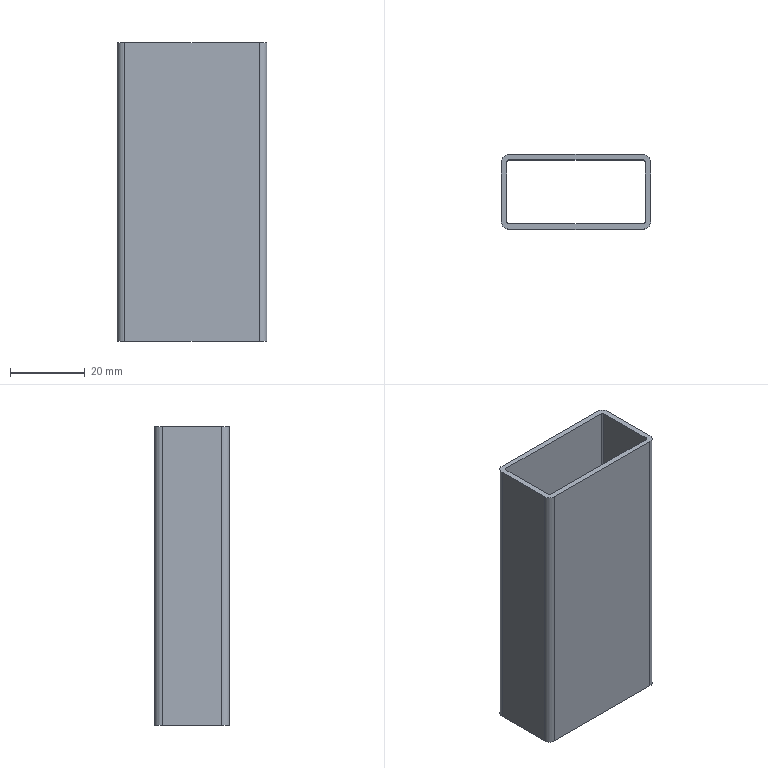Part | STEP file | Q7C0519 | 1 solid | 18 faces | box 40 x 20 x 80 mm | volume 13422 mm3 | plane 10 | cylinder 8 | commonest cylinder face diameters 1 x4 4 x4
STEP:
#1=CARTESIAN_POINT('',(0.,0.,0.));
#2=DIRECTION('',(0.,0.,1.));
#3=DIRECTION('',(1.,0.,0.));
#4=AXIS2_PLACEMENT_3D('',#1,#2,#3);
#5=CARTESIAN_POINT('',(18.,-10.,80.));
#6=VERTEX_POINT('',#5);
#7=CARTESIAN_POINT('',(20.,-8.,80.));
#8=VERTEX_POINT('',#7);
#9=CARTESIAN_POINT('',(18.,-8.,80.));
#10=DIRECTION('',(0.,0.,1.));
#11=DIRECTION('',(1.,0.,0.));
#12=AXIS2_PLACEMENT_3D('',#9,#10,#11);
#13=CIRCLE('',#12,2.);
#14=CARTESIAN_POINT('',(18.,-8.,80.));
#15=DIRECTION('',(0.,0.,1.));
#16=DIRECTION('',(1.,0.,0.));
#17=AXIS2_PLACEMENT_3D('',#14,#15,#16);
#18=PLANE('',#17);
#19=CARTESIAN_POINT('',(0.,0.));
#20=DIRECTION('',(1.,0.));
#21=AXIS2_PLACEMENT_2D('',#19,#20);
#22=CIRCLE('',#21,2.);
#23=(GEOMETRIC_REPRESENTATION_CONTEXT(2)PARAMETRIC_REPRESENTATION_CONTEXT()REPRESENTATION_CONTEXT('',''));
#24=DEFINITIONAL_REPRESENTATION('',(#22),#23);
#25=PCURVE('',#18,#24);
#26=CARTESIAN_POINT('',(18.,-8.,80.));
#27=DIRECTION('',(0.,0.,-1.));
#28=DIRECTION('',(-1.,0.,0.));
#29=AXIS2_PLACEMENT_3D('',#26,#27,#28);
#30=CYLINDRICAL_SURFACE('',#29,2.);
#31=CARTESIAN_POINT('',(9.425,0.));
#32=DIRECTION('',(-1.,0.));
#33=VECTOR('',#32,1.);
#34=LINE('',#31,#33);
#35=(GEOMETRIC_REPRESENTATION_CONTEXT(2)PARAMETRIC_REPRESENTATION_CONTEXT()REPRESENTATION_CONTEXT('',''));
#36=DEFINITIONAL_REPRESENTATION('',(#34),#35);
#37=PCURVE('',#30,#36);
#38=SURFACE_CURVE('',#13,(#25,#37),.PCURVE_S1.);
#39=EDGE_CURVE('',#6,#8,#38,.T.);
#40=ORIENTED_EDGE('',*,*,#39,.T.);
#41=CARTESIAN_POINT('',(20.,8.,80.));
#42=VERTEX_POINT('',#41);
#43=CARTESIAN_POINT('',(20.,8.,80.));
#44=DIRECTION('',(0.,1.,0.));
#45=VECTOR('',#44,1.);
#46=LINE('',#43,#45);
#47=CARTESIAN_POINT('',(2.,16.));
#48=DIRECTION('',(0.,1.));
#49=VECTOR('',#48,1.);
#50=LINE('',#47,#49);
#51=(GEOMETRIC_REPRESENTATION_CONTEXT(2)PARAMETRIC_REPRESENTATION_CONTEXT()REPRESENTATION_CONTEXT('',''));
#52=DEFINITIONAL_REPRESENTATION('',(#50),#51);
#53=PCURVE('',#18,#52);
#54=CARTESIAN_POINT('',(20.,8.,80.));
#55=DIRECTION('',(-1.,0.,0.));
#56=DIRECTION('',(0.,-1.,0.));
#57=AXIS2_PLACEMENT_3D('',#54,#55,#56);
#58=PLANE('',#57);
#59=CARTESIAN_POINT('',(0.,0.));
#60=DIRECTION('',(-1.,0.));
#61=VECTOR('',#60,1.);
#62=LINE('',#59,#61);
#63=(GEOMETRIC_REPRESENTATION_CONTEXT(2)PARAMETRIC_REPRESENTATION_CONTEXT()REPRESENTATION_CONTEXT('',''));
#64=DEFINITIONAL_REPRESENTATION('',(#62),#63);
#65=PCURVE('',#58,#64);
#66=SURFACE_CURVE('',#46,(#53,#65),.PCURVE_S1.);
#67=EDGE_CURVE('',#8,#42,#66,.T.);
#68=ORIENTED_EDGE('',*,*,#67,.T.);
#69=CARTESIAN_POINT('',(18.,10.,80.));
#70=VERTEX_POINT('',#69);
#71=CARTESIAN_POINT('',(18.,8.,80.));
#72=DIRECTION('',(0.,0.,1.));
#73=DIRECTION('',(-1.,0.,0.));
#74=AXIS2_PLACEMENT_3D('',#71,#72,#73);
#75=CIRCLE('',#74,2.);
#76=CARTESIAN_POINT('',(0.,16.));
#77=DIRECTION('',(-1.,0.));
#78=AXIS2_PLACEMENT_2D('',#76,#77);
#79=CIRCLE('',#78,2.);
#80=(GEOMETRIC_REPRESENTATION_CONTEXT(2)PARAMETRIC_REPRESENTATION_CONTEXT()REPRESENTATION_CONTEXT('',''));
#81=DEFINITIONAL_REPRESENTATION('',(#79),#80);
#82=PCURVE('',#18,#81);
#83=CARTESIAN_POINT('',(18.,8.,80.));
#84=DIRECTION('',(0.,0.,-1.));
#85=DIRECTION('',(-1.,0.,0.));
#86=AXIS2_PLACEMENT_3D('',#83,#84,#85);
#87=CYLINDRICAL_SURFACE('',#86,2.);
#88=CARTESIAN_POINT('',(6.283,0.));
#89=DIRECTION('',(-1.,0.));
#90=VECTOR('',#89,1.);
#91=LINE('',#88,#90);
#92=(GEOMETRIC_REPRESENTATION_CONTEXT(2)PARAMETRIC_REPRESENTATION_CONTEXT()REPRESENTATION_CONTEXT('',''));
#93=DEFINITIONAL_REPRESENTATION('',(#91),#92);
#94=PCURVE('',#87,#93);
#95=SURFACE_CURVE('',#75,(#82,#94),.PCURVE_S1.);
#96=EDGE_CURVE('',#42,#70,#95,.T.);
#97=ORIENTED_EDGE('',*,*,#96,.T.);
#98=CARTESIAN_POINT('',(-18.,10.,80.));
#99=VERTEX_POINT('',#98);
#100=CARTESIAN_POINT('',(-18.,10.,80.));
#101=DIRECTION('',(-1.,0.,0.));
#102=VECTOR('',#101,1.);
#103=LINE('',#100,#102);
#104=CARTESIAN_POINT('',(-36.,18.));
#105=DIRECTION('',(-1.,0.));
#106=VECTOR('',#105,1.);
#107=LINE('',#104,#106);
#108=(GEOMETRIC_REPRESENTATION_CONTEXT(2)PARAMETRIC_REPRESENTATION_CONTEXT()REPRESENTATION_CONTEXT('',''));
#109=DEFINITIONAL_REPRESENTATION('',(#107),#108);
#110=PCURVE('',#18,#109);
#111=CARTESIAN_POINT('',(-18.,10.,80.));
#112=DIRECTION('',(0.,-1.,0.));
#113=DIRECTION('',(1.,0.,0.));
#114=AXIS2_PLACEMENT_3D('',#111,#112,#113);
#115=PLANE('',#114);
#116=CARTESIAN_POINT('',(0.,0.));
#117=DIRECTION('',(-1.,0.));
#118=VECTOR('',#117,1.);
#119=LINE('',#116,#118);
#120=(GEOMETRIC_REPRESENTATION_CONTEXT(2)PARAMETRIC_REPRESENTATION_CONTEXT()REPRESENTATION_CONTEXT('',''));
#121=DEFINITIONAL_REPRESENTATION('',(#119),#120);
#122=PCURVE('',#115,#121);
#123=SURFACE_CURVE('',#103,(#110,#122),.PCURVE_S1.);
#124=EDGE_CURVE('',#70,#99,#123,.T.);
#125=ORIENTED_EDGE('',*,*,#124,.T.);
#126=CARTESIAN_POINT('',(-20.,8.,80.));
#127=VERTEX_POINT('',#126);
#128=CARTESIAN_POINT('',(-18.,8.,80.));
#129=DIRECTION('',(0.,0.,1.));
#130=DIRECTION('',(1.,0.,0.));
#131=AXIS2_PLACEMENT_3D('',#128,#129,#130);
#132=CIRCLE('',#131,2.);
#133=CARTESIAN_POINT('',(-36.,16.));
#134=DIRECTION('',(1.,0.));
#135=AXIS2_PLACEMENT_2D('',#133,#134);
#136=CIRCLE('',#135,2.);
#137=(GEOMETRIC_REPRESENTATION_CONTEXT(2)PARAMETRIC_REPRESENTATION_CONTEXT()REPRESENTATION_CONTEXT('',''));
#138=DEFINITIONAL_REPRESENTATION('',(#136),#137);
#139=PCURVE('',#18,#138);
#140=CARTESIAN_POINT('',(-18.,8.,80.));
#141=DIRECTION('',(0.,0.,-1.));
#142=DIRECTION('',(-1.,0.,0.));
#143=AXIS2_PLACEMENT_3D('',#140,#141,#142);
#144=CYLINDRICAL_SURFACE('',#143,2.);
#145=CARTESIAN_POINT('',(3.142,0.));
#146=DIRECTION('',(-1.,0.));
#147=VECTOR('',#146,1.);
#148=LINE('',#145,#147);
#149=(GEOMETRIC_REPRESENTATION_CONTEXT(2)PARAMETRIC_REPRESENTATION_CONTEXT()REPRESENTATION_CONTEXT('',''));
#150=DEFINITIONAL_REPRESENTATION('',(#148),#149);
#151=PCURVE('',#144,#150);
#152=SURFACE_CURVE('',#132,(#139,#151),.PCURVE_S1.);
#153=EDGE_CURVE('',#99,#127,#152,.T.);
#154=ORIENTED_EDGE('',*,*,#153,.T.);
#155=CARTESIAN_POINT('',(-20.,-8.,80.));
#156=VERTEX_POINT('',#155);
#157=CARTESIAN_POINT('',(-20.,8.,80.));
#158=DIRECTION('',(0.,-1.,0.));
#159=VECTOR('',#158,1.);
#160=LINE('',#157,#159);
#161=CARTESIAN_POINT('',(-38.,16.));
#162=DIRECTION('',(0.,-1.));
#163=VECTOR('',#162,1.);
#164=LINE('',#161,#163);
#165=(GEOMETRIC_REPRESENTATION_CONTEXT(2)PARAMETRIC_REPRESENTATION_CONTEXT()REPRESENTATION_CONTEXT('',''));
#166=DEFINITIONAL_REPRESENTATION('',(#164),#165);
#167=PCURVE('',#18,#166);
#168=CARTESIAN_POINT('',(-20.,8.,80.));
#169=DIRECTION('',(1.,0.,0.));
#170=DIRECTION('',(0.,1.,0.));
#171=AXIS2_PLACEMENT_3D('',#168,#169,#170);
#172=PLANE('',#171);
#173=CARTESIAN_POINT('',(0.,0.));
#174=DIRECTION('',(-1.,0.));
#175=VECTOR('',#174,1.);
#176=LINE('',#173,#175);
#177=(GEOMETRIC_REPRESENTATION_CONTEXT(2)PARAMETRIC_REPRESENTATION_CONTEXT()REPRESENTATION_CONTEXT('',''));
#178=DEFINITIONAL_REPRESENTATION('',(#176),#177);
#179=PCURVE('',#172,#178);
#180=SURFACE_CURVE('',#160,(#167,#179),.PCURVE_S1.);
#181=EDGE_CURVE('',#127,#156,#180,.T.);
#182=ORIENTED_EDGE('',*,*,#181,.T.);
#183=CARTESIAN_POINT('',(-18.,-10.,80.));
#184=VERTEX_POINT('',#183);
#185=CARTESIAN_POINT('',(-18.,-8.,80.));
#186=DIRECTION('',(0.,0.,1.));
#187=DIRECTION('',(1.,0.,0.));
#188=AXIS2_PLACEMENT_3D('',#185,#186,#187);
#189=CIRCLE('',#188,2.);
#190=CARTESIAN_POINT('',(-36.,0.));
#191=DIRECTION('',(1.,0.));
#192=AXIS2_PLACEMENT_2D('',#190,#191);
#193=CIRCLE('',#192,2.);
#194=(GEOMETRIC_REPRESENTATION_CONTEXT(2)PARAMETRIC_REPRESENTATION_CONTEXT()REPRESENTATION_CONTEXT('',''));
#195=DEFINITIONAL_REPRESENTATION('',(#193),#194);
#196=PCURVE('',#18,#195);
#197=CARTESIAN_POINT('',(-18.,-8.,80.));
#198=DIRECTION('',(0.,0.,-1.));
#199=DIRECTION('',(-1.,0.,0.));
#200=AXIS2_PLACEMENT_3D('',#197,#198,#199);
#201=CYLINDRICAL_SURFACE('',#200,2.);
#202=CARTESIAN_POINT('',(9.425,0.));
#203=DIRECTION('',(-1.,0.));
#204=VECTOR('',#203,1.);
#205=LINE('',#202,#204);
#206=(GEOMETRIC_REPRESENTATION_CONTEXT(2)PARAMETRIC_REPRESENTATION_CONTEXT()REPRESENTATION_CONTEXT('',''));
#207=DEFINITIONAL_REPRESENTATION('',(#205),#206);
#208=PCURVE('',#201,#207);
#209=SURFACE_CURVE('',#189,(#196,#208),.PCURVE_S1.);
#210=EDGE_CURVE('',#156,#184,#209,.T.);
#211=ORIENTED_EDGE('',*,*,#210,.T.);
#212=CARTESIAN_POINT('',(-18.,-10.,80.));
#213=DIRECTION('',(1.,0.,0.));
#214=VECTOR('',#213,1.);
#215=LINE('',#212,#214);
#216=CARTESIAN_POINT('',(-36.,-2.));
#217=DIRECTION('',(1.,0.));
#218=VECTOR('',#217,1.);
#219=LINE('',#216,#218);
#220=(GEOMETRIC_REPRESENTATION_CONTEXT(2)PARAMETRIC_REPRESENTATION_CONTEXT()REPRESENTATION_CONTEXT('',''));
#221=DEFINITIONAL_REPRESENTATION('',(#219),#220);
#222=PCURVE('',#18,#221);
#223=CARTESIAN_POINT('',(-18.,-10.,80.));
#224=DIRECTION('',(0.,1.,0.));
#225=DIRECTION('',(0.,0.,1.));
#226=AXIS2_PLACEMENT_3D('',#223,#224,#225);
#227=PLANE('',#226);
#228=CARTESIAN_POINT('',(0.,0.));
#229=DIRECTION('',(0.,1.));
#230=VECTOR('',#229,1.);
#231=LINE('',#228,#230);
#232=(GEOMETRIC_REPRESENTATION_CONTEXT(2)PARAMETRIC_REPRESENTATION_CONTEXT()REPRESENTATION_CONTEXT('',''));
#233=DEFINITIONAL_REPRESENTATION('',(#231),#232);
#234=PCURVE('',#227,#233);
#235=SURFACE_CURVE('',#215,(#222,#234),.PCURVE_S1.);
#236=EDGE_CURVE('',#184,#6,#235,.T.);
#237=ORIENTED_EDGE('',*,*,#236,.T.);
#238=EDGE_LOOP('',(#40,#68,#97,#125,#154,#182,#211,#237));
#239=FACE_BOUND('',#238,.T.);
#240=CARTESIAN_POINT('',(18.,8.5,80.));
#241=VERTEX_POINT('',#240);
#242=CARTESIAN_POINT('',(-18.,8.5,80.));
#243=VERTEX_POINT('',#242);
#244=CARTESIAN_POINT('',(-18.,8.5,80.));
#245=DIRECTION('',(-1.,0.,0.));
#246=VECTOR('',#245,1.);
#247=LINE('',#244,#246);
#248=CARTESIAN_POINT('',(-36.,16.5));
#249=DIRECTION('',(-1.,0.));
#250=VECTOR('',#249,1.);
#251=LINE('',#248,#250);
#252=(GEOMETRIC_REPRESENTATION_CONTEXT(2)PARAMETRIC_REPRESENTATION_CONTEXT()REPRESENTATION_CONTEXT('',''));
#253=DEFINITIONAL_REPRESENTATION('',(#251),#252);
#254=PCURVE('',#18,#253);
#255=CARTESIAN_POINT('',(-18.,8.5,80.));
#256=DIRECTION('',(0.,-1.,0.));
#257=DIRECTION('',(1.,0.,0.));
#258=AXIS2_PLACEMENT_3D('',#255,#256,#257);
#259=PLANE('',#258);
#260=CARTESIAN_POINT('',(0.,0.));
#261=DIRECTION('',(-1.,0.));
#262=VECTOR('',#261,1.);
#263=LINE('',#260,#262);
#264=(GEOMETRIC_REPRESENTATION_CONTEXT(2)PARAMETRIC_REPRESENTATION_CONTEXT()REPRESENTATION_CONTEXT('',''));
#265=DEFINITIONAL_REPRESENTATION('',(#263),#264);
#266=PCURVE('',#259,#265);
#267=SURFACE_CURVE('',#247,(#254,#266),.PCURVE_S1.);
#268=EDGE_CURVE('',#241,#243,#267,.T.);
#269=ORIENTED_EDGE('',*,*,#268,.F.);
#270=CARTESIAN_POINT('',(18.5,8.,80.));
#271=VERTEX_POINT('',#270);
#272=CARTESIAN_POINT('',(18.,8.,80.));
#273=DIRECTION('',(0.,0.,1.));
#274=DIRECTION('',(-1.,0.,0.));
#275=AXIS2_PLACEMENT_3D('',#272,#273,#274);
#276=CIRCLE('',#275,0.5);
#277=CARTESIAN_POINT('',(0.,16.));
#278=DIRECTION('',(-1.,0.));
#279=AXIS2_PLACEMENT_2D('',#277,#278);
#280=CIRCLE('',#279,0.5);
#281=(GEOMETRIC_REPRESENTATION_CONTEXT(2)PARAMETRIC_REPRESENTATION_CONTEXT()REPRESENTATION_CONTEXT('',''));
#282=DEFINITIONAL_REPRESENTATION('',(#280),#281);
#283=PCURVE('',#18,#282);
#284=CARTESIAN_POINT('',(18.,8.,80.));
#285=DIRECTION('',(0.,0.,-1.));
#286=DIRECTION('',(-1.,0.,0.));
#287=AXIS2_PLACEMENT_3D('',#284,#285,#286);
#288=CYLINDRICAL_SURFACE('',#287,0.5);
#289=CARTESIAN_POINT('',(6.283,0.));
#290=DIRECTION('',(-1.,0.));
#291=VECTOR('',#290,1.);
#292=LINE('',#289,#291);
#293=(GEOMETRIC_REPRESENTATION_CONTEXT(2)PARAMETRIC_REPRESENTATION_CONTEXT()REPRESENTATION_CONTEXT('',''));
#294=DEFINITIONAL_REPRESENTATION('',(#292),#293);
#295=PCURVE('',#288,#294);
#296=SURFACE_CURVE('',#276,(#283,#295),.PCURVE_S1.);
#297=EDGE_CURVE('',#271,#241,#296,.T.);
#298=ORIENTED_EDGE('',*,*,#297,.F.);
#299=CARTESIAN_POINT('',(18.5,-8.,80.));
#300=VERTEX_POINT('',#299);
#301=CARTESIAN_POINT('',(18.5,8.,80.));
#302=DIRECTION('',(0.,1.,0.));
#303=VECTOR('',#302,1.);
#304=LINE('',#301,#303);
#305=CARTESIAN_POINT('',(0.5,16.));
#306=DIRECTION('',(0.,1.));
#307=VECTOR('',#306,1.);
#308=LINE('',#305,#307);
#309=(GEOMETRIC_REPRESENTATION_CONTEXT(2)PARAMETRIC_REPRESENTATION_CONTEXT()REPRESENTATION_CONTEXT('',''));
#310=DEFINITIONAL_REPRESENTATION('',(#308),#309);
#311=PCURVE('',#18,#310);
#312=CARTESIAN_POINT('',(18.5,8.,80.));
#313=DIRECTION('',(-1.,0.,0.));
#314=DIRECTION('',(0.,0.,1.));
#315=AXIS2_PLACEMENT_3D('',#312,#313,#314);
#316=PLANE('',#315);
#317=CARTESIAN_POINT('',(0.,0.));
#318=DIRECTION('',(0.,1.));
#319=VECTOR('',#318,1.);
#320=LINE('',#317,#319);
#321=(GEOMETRIC_REPRESENTATION_CONTEXT(2)PARAMETRIC_REPRESENTATION_CONTEXT()REPRESENTATION_CONTEXT('',''));
#322=DEFINITIONAL_REPRESENTATION('',(#320),#321);
#323=PCURVE('',#316,#322);
#324=SURFACE_CURVE('',#304,(#311,#323),.PCURVE_S1.);
#325=EDGE_CURVE('',#300,#271,#324,.T.);
#326=ORIENTED_EDGE('',*,*,#325,.F.);
#327=CARTESIAN_POINT('',(18.,-8.5,80.));
#328=VERTEX_POINT('',#327);
#329=CARTESIAN_POINT('',(18.,-8.,80.));
#330=DIRECTION('',(0.,0.,1.));
#331=DIRECTION('',(1.,0.,0.));
#332=AXIS2_PLACEMENT_3D('',#329,#330,#331);
#333=CIRCLE('',#332,0.5);
#334=CARTESIAN_POINT('',(0.,0.));
#335=DIRECTION('',(1.,0.));
#336=AXIS2_PLACEMENT_2D('',#334,#335);
#337=CIRCLE('',#336,0.5);
#338=(GEOMETRIC_REPRESENTATION_CONTEXT(2)PARAMETRIC_REPRESENTATION_CONTEXT()REPRESENTATION_CONTEXT('',''));
#339=DEFINITIONAL_REPRESENTATION('',(#337),#338);
#340=PCURVE('',#18,#339);
#341=CARTESIAN_POINT('',(18.,-8.,80.));
#342=DIRECTION('',(0.,0.,-1.));
#343=DIRECTION('',(-1.,0.,0.));
#344=AXIS2_PLACEMENT_3D('',#341,#342,#343);
#345=CYLINDRICAL_SURFACE('',#344,0.5);
#346=CARTESIAN_POINT('',(9.425,0.));
#347=DIRECTION('',(-1.,0.));
#348=VECTOR('',#347,1.);
#349=LINE('',#346,#348);
#350=(GEOMETRIC_REPRESENTATION_CONTEXT(2)PARAMETRIC_REPRESENTATION_CONTEXT()REPRESENTATION_CONTEXT('',''));
#351=DEFINITIONAL_REPRESENTATION('',(#349),#350);
#352=PCURVE('',#345,#351);
#353=SURFACE_CURVE('',#333,(#340,#352),.PCURVE_S1.);
#354=EDGE_CURVE('',#328,#300,#353,.T.);
#355=ORIENTED_EDGE('',*,*,#354,.F.);
#356=CARTESIAN_POINT('',(-18.,-8.5,80.));
#357=VERTEX_POINT('',#356);
#358=CARTESIAN_POINT('',(-18.,-8.5,80.));
#359=DIRECTION('',(1.,0.,0.));
#360=VECTOR('',#359,1.);
#361=LINE('',#358,#360);
#362=CARTESIAN_POINT('',(-36.,-0.5));
#363=DIRECTION('',(1.,0.));
#364=VECTOR('',#363,1.);
#365=LINE('',#362,#364);
#366=(GEOMETRIC_REPRESENTATION_CONTEXT(2)PARAMETRIC_REPRESENTATION_CONTEXT()REPRESENTATION_CONTEXT('',''));
#367=DEFINITIONAL_REPRESENTATION('',(#365),#366);
#368=PCURVE('',#18,#367);
#369=CARTESIAN_POINT('',(-18.,-8.5,80.));
#370=DIRECTION('',(0.,1.,0.));
#371=DIRECTION('',(-1.,0.,0.));
#372=AXIS2_PLACEMENT_3D('',#369,#370,#371);
#373=PLANE('',#372);
#374=CARTESIAN_POINT('',(0.,0.));
#375=DIRECTION('',(-1.,0.));
#376=VECTOR('',#375,1.);
#377=LINE('',#374,#376);
#378=(GEOMETRIC_REPRESENTATION_CONTEXT(2)PARAMETRIC_REPRESENTATION_CONTEXT()REPRESENTATION_CONTEXT('',''));
#379=DEFINITIONAL_REPRESENTATION('',(#377),#378);
#380=PCURVE('',#373,#379);
#381=SURFACE_CURVE('',#361,(#368,#380),.PCURVE_S1.);
#382=EDGE_CURVE('',#357,#328,#381,.T.);
#383=ORIENTED_EDGE('',*,*,#382,.F.);
#384=CARTESIAN_POINT('',(-18.5,-8.,80.));
#385=VERTEX_POINT('',#384);
#386=CARTESIAN_POINT('',(-18.,-8.,80.));
#387=DIRECTION('',(0.,0.,1.));
#388=DIRECTION('',(1.,0.,0.));
#389=AXIS2_PLACEMENT_3D('',#386,#387,#388);
#390=CIRCLE('',#389,0.5);
#391=CARTESIAN_POINT('',(-36.,0.));
#392=DIRECTION('',(1.,0.));
#393=AXIS2_PLACEMENT_2D('',#391,#392);
#394=CIRCLE('',#393,0.5);
#395=(GEOMETRIC_REPRESENTATION_CONTEXT(2)PARAMETRIC_REPRESENTATION_CONTEXT()REPRESENTATION_CONTEXT('',''));
#396=DEFINITIONAL_REPRESENTATION('',(#394),#395);
#397=PCURVE('',#18,#396);
#398=CARTESIAN_POINT('',(-18.,-8.,80.));
#399=DIRECTION('',(0.,0.,-1.));
#400=DIRECTION('',(-1.,0.,0.));
#401=AXIS2_PLACEMENT_3D('',#398,#399,#400);
#402=CYLINDRICAL_SURFACE('',#401,0.5);
#403=CARTESIAN_POINT('',(9.425,0.));
#404=DIRECTION('',(-1.,0.));
#405=VECTOR('',#404,1.);
#406=LINE('',#403,#405);
#407=(GEOMETRIC_REPRESENTATION_CONTEXT(2)PARAMETRIC_REPRESENTATION_CONTEXT()REPRESENTATION_CONTEXT('',''));
#408=DEFINITIONAL_REPRESENTATION('',(#406),#407);
#409=PCURVE('',#402,#408);
#410=SURFACE_CURVE('',#390,(#397,#409),.PCURVE_S1.);
#411=EDGE_CURVE('',#385,#357,#410,.T.);
#412=ORIENTED_EDGE('',*,*,#411,.F.);
#413=CARTESIAN_POINT('',(-18.5,8.,80.));
#414=VERTEX_POINT('',#413);
#415=CARTESIAN_POINT('',(-18.5,8.,80.));
#416=DIRECTION('',(0.,-1.,0.));
#417=VECTOR('',#416,1.);
#418=LINE('',#415,#417);
#419=CARTESIAN_POINT('',(-36.5,16.));
#420=DIRECTION('',(0.,-1.));
#421=VECTOR('',#420,1.);
#422=LINE('',#419,#421);
#423=(GEOMETRIC_REPRESENTATION_CONTEXT(2)PARAMETRIC_REPRESENTATION_CONTEXT()REPRESENTATION_CONTEXT('',''));
#424=DEFINITIONAL_REPRESENTATION('',(#422),#423);
#425=PCURVE('',#18,#424);
#426=CARTESIAN_POINT('',(-18.5,8.,80.));
#427=DIRECTION('',(1.,0.,0.));
#428=DIRECTION('',(0.,0.,-1.));
#429=AXIS2_PLACEMENT_3D('',#426,#427,#428);
#430=PLANE('',#429);
#431=CARTESIAN_POINT('',(0.,0.));
#432=DIRECTION('',(0.,-1.));
#433=VECTOR('',#432,1.);
#434=LINE('',#431,#433);
#435=(GEOMETRIC_REPRESENTATION_CONTEXT(2)PARAMETRIC_REPRESENTATION_CONTEXT()REPRESENTATION_CONTEXT('',''));
#436=DEFINITIONAL_REPRESENTATION('',(#434),#435);
#437=PCURVE('',#430,#436);
#438=SURFACE_CURVE('',#418,(#425,#437),.PCURVE_S1.);
#439=EDGE_CURVE('',#414,#385,#438,.T.);
#440=ORIENTED_EDGE('',*,*,#439,.F.);
#441=CARTESIAN_POINT('',(-18.,8.,80.));
#442=DIRECTION('',(0.,0.,1.));
#443=DIRECTION('',(1.,0.,0.));
#444=AXIS2_PLACEMENT_3D('',#441,#442,#443);
#445=CIRCLE('',#444,0.5);
#446=CARTESIAN_POINT('',(-36.,16.));
#447=DIRECTION('',(1.,0.));
#448=AXIS2_PLACEMENT_2D('',#446,#447);
#449=CIRCLE('',#448,0.5);
#450=(GEOMETRIC_REPRESENTATION_CONTEXT(2)PARAMETRIC_REPRESENTATION_CONTEXT()REPRESENTATION_CONTEXT('',''));
#451=DEFINITIONAL_REPRESENTATION('',(#449),#450);
#452=PCURVE('',#18,#451);
#453=CARTESIAN_POINT('',(-18.,8.,80.));
#454=DIRECTION('',(0.,0.,-1.));
#455=DIRECTION('',(-1.,0.,0.));
#456=AXIS2_PLACEMENT_3D('',#453,#454,#455);
#457=CYLINDRICAL_SURFACE('',#456,0.5);
#458=CARTESIAN_POINT('',(3.142,0.));
#459=DIRECTION('',(-1.,0.));
#460=VECTOR('',#459,1.);
#461=LINE('',#458,#460);
#462=(GEOMETRIC_REPRESENTATION_CONTEXT(2)PARAMETRIC_REPRESENTATION_CONTEXT()REPRESENTATION_CONTEXT('',''));
#463=DEFINITIONAL_REPRESENTATION('',(#461),#462);
#464=PCURVE('',#457,#463);
#465=SURFACE_CURVE('',#445,(#452,#464),.PCURVE_S1.);
#466=EDGE_CURVE('',#243,#414,#465,.T.);
#467=ORIENTED_EDGE('',*,*,#466,.F.);
#468=EDGE_LOOP('',(#269,#298,#326,#355,#383,#412,#440,#467));
#469=FACE_BOUND('',#468,.T.);
#470=ADVANCED_FACE('',(#239,#469),#18,.T.);
#471=CARTESIAN_POINT('',(18.,-10.,0.));
#472=VERTEX_POINT('',#471);
#473=CARTESIAN_POINT('',(20.,-8.,0.));
#474=VERTEX_POINT('',#473);
#475=CARTESIAN_POINT('',(18.,-8.,0.));
#476=DIRECTION('',(0.,0.,1.));
#477=DIRECTION('',(1.,0.,0.));
#478=AXIS2_PLACEMENT_3D('',#475,#476,#477);
#479=CIRCLE('',#478,2.);
#480=CARTESIAN_POINT('',(18.,-8.,0.));
#481=DIRECTION('',(0.,0.,1.));
#482=DIRECTION('',(1.,0.,0.));
#483=AXIS2_PLACEMENT_3D('',#480,#481,#482);
#484=PLANE('',#483);
#485=CARTESIAN_POINT('',(0.,0.));
#486=DIRECTION('',(1.,0.));
#487=AXIS2_PLACEMENT_2D('',#485,#486);
#488=CIRCLE('',#487,2.);
#489=(GEOMETRIC_REPRESENTATION_CONTEXT(2)PARAMETRIC_REPRESENTATION_CONTEXT()REPRESENTATION_CONTEXT('',''));
#490=DEFINITIONAL_REPRESENTATION('',(#488),#489);
#491=PCURVE('',#484,#490);
#492=CARTESIAN_POINT('',(9.425,80.));
#493=DIRECTION('',(-1.,0.));
#494=VECTOR('',#493,1.);
#495=LINE('',#492,#494);
#496=(GEOMETRIC_REPRESENTATION_CONTEXT(2)PARAMETRIC_REPRESENTATION_CONTEXT()REPRESENTATION_CONTEXT('',''));
#497=DEFINITIONAL_REPRESENTATION('',(#495),#496);
#498=PCURVE('',#30,#497);
#499=SURFACE_CURVE('',#479,(#491,#498),.PCURVE_S1.);
#500=EDGE_CURVE('',#472,#474,#499,.T.);
#501=ORIENTED_EDGE('',*,*,#500,.F.);
#502=CARTESIAN_POINT('',(-18.,-10.,0.));
#503=VERTEX_POINT('',#502);
#504=CARTESIAN_POINT('',(-18.,-10.,0.));
#505=DIRECTION('',(1.,0.,0.));
#506=VECTOR('',#505,1.);
#507=LINE('',#504,#506);
#508=CARTESIAN_POINT('',(-36.,-2.));
#509=DIRECTION('',(1.,0.));
#510=VECTOR('',#509,1.);
#511=LINE('',#508,#510);
#512=(GEOMETRIC_REPRESENTATION_CONTEXT(2)PARAMETRIC_REPRESENTATION_CONTEXT()REPRESENTATION_CONTEXT('',''));
#513=DEFINITIONAL_REPRESENTATION('',(#511),#512);
#514=PCURVE('',#484,#513);
#515=CARTESIAN_POINT('',(-80.,0.));
#516=DIRECTION('',(0.,1.));
#517=VECTOR('',#516,1.);
#518=LINE('',#515,#517);
#519=(GEOMETRIC_REPRESENTATION_CONTEXT(2)PARAMETRIC_REPRESENTATION_CONTEXT()REPRESENTATION_CONTEXT('',''));
#520=DEFINITIONAL_REPRESENTATION('',(#518),#519);
#521=PCURVE('',#227,#520);
#522=SURFACE_CURVE('',#507,(#514,#521),.PCURVE_S1.);
#523=EDGE_CURVE('',#503,#472,#522,.T.);
#524=ORIENTED_EDGE('',*,*,#523,.F.);
#525=CARTESIAN_POINT('',(-20.,-8.,0.));
#526=VERTEX_POINT('',#525);
#527=CARTESIAN_POINT('',(-18.,-8.,0.));
#528=DIRECTION('',(0.,0.,1.));
#529=DIRECTION('',(1.,0.,0.));
#530=AXIS2_PLACEMENT_3D('',#527,#528,#529);
#531=CIRCLE('',#530,2.);
#532=CARTESIAN_POINT('',(-36.,0.));
#533=DIRECTION('',(1.,0.));
#534=AXIS2_PLACEMENT_2D('',#532,#533);
#535=CIRCLE('',#534,2.);
#536=(GEOMETRIC_REPRESENTATION_CONTEXT(2)PARAMETRIC_REPRESENTATION_CONTEXT()REPRESENTATION_CONTEXT('',''));
#537=DEFINITIONAL_REPRESENTATION('',(#535),#536);
#538=PCURVE('',#484,#537);
#539=CARTESIAN_POINT('',(9.425,80.));
#540=DIRECTION('',(-1.,0.));
#541=VECTOR('',#540,1.);
#542=LINE('',#539,#541);
#543=(GEOMETRIC_REPRESENTATION_CONTEXT(2)PARAMETRIC_REPRESENTATION_CONTEXT()REPRESENTATION_CONTEXT('',''));
#544=DEFINITIONAL_REPRESENTATION('',(#542),#543);
#545=PCURVE('',#201,#544);
#546=SURFACE_CURVE('',#531,(#538,#545),.PCURVE_S1.);
#547=EDGE_CURVE('',#526,#503,#546,.T.);
#548=ORIENTED_EDGE('',*,*,#547,.F.);
#549=CARTESIAN_POINT('',(-20.,8.,0.));
#550=VERTEX_POINT('',#549);
#551=CARTESIAN_POINT('',(-20.,8.,0.));
#552=DIRECTION('',(0.,-1.,0.));
#553=VECTOR('',#552,1.);
#554=LINE('',#551,#553);
#555=CARTESIAN_POINT('',(-38.,16.));
#556=DIRECTION('',(0.,-1.));
#557=VECTOR('',#556,1.);
#558=LINE('',#555,#557);
#559=(GEOMETRIC_REPRESENTATION_CONTEXT(2)PARAMETRIC_REPRESENTATION_CONTEXT()REPRESENTATION_CONTEXT('',''));
#560=DEFINITIONAL_REPRESENTATION('',(#558),#559);
#561=PCURVE('',#484,#560);
#562=CARTESIAN_POINT('',(0.,-80.));
#563=DIRECTION('',(-1.,0.));
#564=VECTOR('',#563,1.);
#565=LINE('',#562,#564);
#566=(GEOMETRIC_REPRESENTATION_CONTEXT(2)PARAMETRIC_REPRESENTATION_CONTEXT()REPRESENTATION_CONTEXT('',''));
#567=DEFINITIONAL_REPRESENTATION('',(#565),#566);
#568=PCURVE('',#172,#567);
#569=SURFACE_CURVE('',#554,(#561,#568),.PCURVE_S1.);
#570=EDGE_CURVE('',#550,#526,#569,.T.);
#571=ORIENTED_EDGE('',*,*,#570,.F.);
#572=CARTESIAN_POINT('',(-18.,10.,0.));
#573=VERTEX_POINT('',#572);
#574=CARTESIAN_POINT('',(-18.,8.,0.));
#575=DIRECTION('',(0.,0.,1.));
#576=DIRECTION('',(1.,0.,0.));
#577=AXIS2_PLACEMENT_3D('',#574,#575,#576);
#578=CIRCLE('',#577,2.);
#579=CARTESIAN_POINT('',(-36.,16.));
#580=DIRECTION('',(1.,0.));
#581=AXIS2_PLACEMENT_2D('',#579,#580);
#582=CIRCLE('',#581,2.);
#583=(GEOMETRIC_REPRESENTATION_CONTEXT(2)PARAMETRIC_REPRESENTATION_CONTEXT()REPRESENTATION_CONTEXT('',''));
#584=DEFINITIONAL_REPRESENTATION('',(#582),#583);
#585=PCURVE('',#484,#584);
#586=CARTESIAN_POINT('',(3.142,80.));
#587=DIRECTION('',(-1.,0.));
#588=VECTOR('',#587,1.);
#589=LINE('',#586,#588);
#590=(GEOMETRIC_REPRESENTATION_CONTEXT(2)PARAMETRIC_REPRESENTATION_CONTEXT()REPRESENTATION_CONTEXT('',''));
#591=DEFINITIONAL_REPRESENTATION('',(#589),#590);
#592=PCURVE('',#144,#591);
#593=SURFACE_CURVE('',#578,(#585,#592),.PCURVE_S1.);
#594=EDGE_CURVE('',#573,#550,#593,.T.);
#595=ORIENTED_EDGE('',*,*,#594,.F.);
#596=CARTESIAN_POINT('',(18.,10.,0.));
#597=VERTEX_POINT('',#596);
#598=CARTESIAN_POINT('',(-18.,10.,0.));
#599=DIRECTION('',(-1.,0.,0.));
#600=VECTOR('',#599,1.);
#601=LINE('',#598,#600);
#602=CARTESIAN_POINT('',(-36.,18.));
#603=DIRECTION('',(-1.,0.));
#604=VECTOR('',#603,1.);
#605=LINE('',#602,#604);
#606=(GEOMETRIC_REPRESENTATION_CONTEXT(2)PARAMETRIC_REPRESENTATION_CONTEXT()REPRESENTATION_CONTEXT('',''));
#607=DEFINITIONAL_REPRESENTATION('',(#605),#606);
#608=PCURVE('',#484,#607);
#609=CARTESIAN_POINT('',(0.,-80.));
#610=DIRECTION('',(-1.,0.));
#611=VECTOR('',#610,1.);
#612=LINE('',#609,#611);
#613=(GEOMETRIC_REPRESENTATION_CONTEXT(2)PARAMETRIC_REPRESENTATION_CONTEXT()REPRESENTATION_CONTEXT('',''));
#614=DEFINITIONAL_REPRESENTATION('',(#612),#613);
#615=PCURVE('',#115,#614);
#616=SURFACE_CURVE('',#601,(#608,#615),.PCURVE_S1.);
#617=EDGE_CURVE('',#597,#573,#616,.T.);
#618=ORIENTED_EDGE('',*,*,#617,.F.);
#619=CARTESIAN_POINT('',(20.,8.,0.));
#620=VERTEX_POINT('',#619);
#621=CARTESIAN_POINT('',(18.,8.,0.));
#622=DIRECTION('',(0.,0.,1.));
#623=DIRECTION('',(-1.,0.,0.));
#624=AXIS2_PLACEMENT_3D('',#621,#622,#623);
#625=CIRCLE('',#624,2.);
#626=CARTESIAN_POINT('',(0.,16.));
#627=DIRECTION('',(-1.,0.));
#628=AXIS2_PLACEMENT_2D('',#626,#627);
#629=CIRCLE('',#628,2.);
#630=(GEOMETRIC_REPRESENTATION_CONTEXT(2)PARAMETRIC_REPRESENTATION_CONTEXT()REPRESENTATION_CONTEXT('',''));
#631=DEFINITIONAL_REPRESENTATION('',(#629),#630);
#632=PCURVE('',#484,#631);
#633=CARTESIAN_POINT('',(6.283,80.));
#634=DIRECTION('',(-1.,0.));
#635=VECTOR('',#634,1.);
#636=LINE('',#633,#635);
#637=(GEOMETRIC_REPRESENTATION_CONTEXT(2)PARAMETRIC_REPRESENTATION_CONTEXT()REPRESENTATION_CONTEXT('',''));
#638=DEFINITIONAL_REPRESENTATION('',(#636),#637);
#639=PCURVE('',#87,#638);
#640=SURFACE_CURVE('',#625,(#632,#639),.PCURVE_S1.);
#641=EDGE_CURVE('',#620,#597,#640,.T.);
#642=ORIENTED_EDGE('',*,*,#641,.F.);
#643=CARTESIAN_POINT('',(20.,8.,0.));
#644=DIRECTION('',(0.,1.,0.));
#645=VECTOR('',#644,1.);
#646=LINE('',#643,#645);
#647=CARTESIAN_POINT('',(2.,16.));
#648=DIRECTION('',(0.,1.));
#649=VECTOR('',#648,1.);
#650=LINE('',#647,#649);
#651=(GEOMETRIC_REPRESENTATION_CONTEXT(2)PARAMETRIC_REPRESENTATION_CONTEXT()REPRESENTATION_CONTEXT('',''));
#652=DEFINITIONAL_REPRESENTATION('',(#650),#651);
#653=PCURVE('',#484,#652);
#654=CARTESIAN_POINT('',(0.,-80.));
#655=DIRECTION('',(-1.,0.));
#656=VECTOR('',#655,1.);
#657=LINE('',#654,#656);
#658=(GEOMETRIC_REPRESENTATION_CONTEXT(2)PARAMETRIC_REPRESENTATION_CONTEXT()REPRESENTATION_CONTEXT('',''));
#659=DEFINITIONAL_REPRESENTATION('',(#657),#658);
#660=PCURVE('',#58,#659);
#661=SURFACE_CURVE('',#646,(#653,#660),.PCURVE_S1.);
#662=EDGE_CURVE('',#474,#620,#661,.T.);
#663=ORIENTED_EDGE('',*,*,#662,.F.);
#664=EDGE_LOOP('',(#501,#524,#548,#571,#595,#618,#642,#663));
#665=FACE_BOUND('',#664,.T.);
#666=CARTESIAN_POINT('',(18.5,8.,0.));
#667=VERTEX_POINT('',#666);
#668=CARTESIAN_POINT('',(18.,8.5,0.));
#669=VERTEX_POINT('',#668);
#670=CARTESIAN_POINT('',(18.,8.,0.));
#671=DIRECTION('',(0.,0.,1.));
#672=DIRECTION('',(-1.,0.,0.));
#673=AXIS2_PLACEMENT_3D('',#670,#671,#672);
#674=CIRCLE('',#673,0.5);
#675=CARTESIAN_POINT('',(0.,16.));
#676=DIRECTION('',(-1.,0.));
#677=AXIS2_PLACEMENT_2D('',#675,#676);
#678=CIRCLE('',#677,0.5);
#679=(GEOMETRIC_REPRESENTATION_CONTEXT(2)PARAMETRIC_REPRESENTATION_CONTEXT()REPRESENTATION_CONTEXT('',''));
#680=DEFINITIONAL_REPRESENTATION('',(#678),#679);
#681=PCURVE('',#484,#680);
#682=CARTESIAN_POINT('',(6.283,80.));
#683=DIRECTION('',(-1.,0.));
#684=VECTOR('',#683,1.);
#685=LINE('',#682,#684);
#686=(GEOMETRIC_REPRESENTATION_CONTEXT(2)PARAMETRIC_REPRESENTATION_CONTEXT()REPRESENTATION_CONTEXT('',''));
#687=DEFINITIONAL_REPRESENTATION('',(#685),#686);
#688=PCURVE('',#288,#687);
#689=SURFACE_CURVE('',#674,(#681,#688),.PCURVE_S1.);
#690=EDGE_CURVE('',#667,#669,#689,.T.);
#691=ORIENTED_EDGE('',*,*,#690,.T.);
#692=CARTESIAN_POINT('',(-18.,8.5,0.));
#693=VERTEX_POINT('',#692);
#694=CARTESIAN_POINT('',(-18.,8.5,0.));
#695=DIRECTION('',(-1.,0.,0.));
#696=VECTOR('',#695,1.);
#697=LINE('',#694,#696);
#698=CARTESIAN_POINT('',(-36.,16.5));
#699=DIRECTION('',(-1.,0.));
#700=VECTOR('',#699,1.);
#701=LINE('',#698,#700);
#702=(GEOMETRIC_REPRESENTATION_CONTEXT(2)PARAMETRIC_REPRESENTATION_CONTEXT()REPRESENTATION_CONTEXT('',''));
#703=DEFINITIONAL_REPRESENTATION('',(#701),#702);
#704=PCURVE('',#484,#703);
#705=CARTESIAN_POINT('',(0.,-80.));
#706=DIRECTION('',(-1.,0.));
#707=VECTOR('',#706,1.);
#708=LINE('',#705,#707);
#709=(GEOMETRIC_REPRESENTATION_CONTEXT(2)PARAMETRIC_REPRESENTATION_CONTEXT()REPRESENTATION_CONTEXT('',''));
#710=DEFINITIONAL_REPRESENTATION('',(#708),#709);
#711=PCURVE('',#259,#710);
#712=SURFACE_CURVE('',#697,(#704,#711),.PCURVE_S1.);
#713=EDGE_CURVE('',#669,#693,#712,.T.);
#714=ORIENTED_EDGE('',*,*,#713,.T.);
#715=CARTESIAN_POINT('',(-18.5,8.,0.));
#716=VERTEX_POINT('',#715);
#717=CARTESIAN_POINT('',(-18.,8.,0.));
#718=DIRECTION('',(0.,0.,1.));
#719=DIRECTION('',(1.,0.,0.));
#720=AXIS2_PLACEMENT_3D('',#717,#718,#719);
#721=CIRCLE('',#720,0.5);
#722=CARTESIAN_POINT('',(-36.,16.));
#723=DIRECTION('',(1.,0.));
#724=AXIS2_PLACEMENT_2D('',#722,#723);
#725=CIRCLE('',#724,0.5);
#726=(GEOMETRIC_REPRESENTATION_CONTEXT(2)PARAMETRIC_REPRESENTATION_CONTEXT()REPRESENTATION_CONTEXT('',''));
#727=DEFINITIONAL_REPRESENTATION('',(#725),#726);
#728=PCURVE('',#484,#727);
#729=CARTESIAN_POINT('',(3.142,80.));
#730=DIRECTION('',(-1.,0.));
#731=VECTOR('',#730,1.);
#732=LINE('',#729,#731);
#733=(GEOMETRIC_REPRESENTATION_CONTEXT(2)PARAMETRIC_REPRESENTATION_CONTEXT()REPRESENTATION_CONTEXT('',''));
#734=DEFINITIONAL_REPRESENTATION('',(#732),#733);
#735=PCURVE('',#457,#734);
#736=SURFACE_CURVE('',#721,(#728,#735),.PCURVE_S1.);
#737=EDGE_CURVE('',#693,#716,#736,.T.);
#738=ORIENTED_EDGE('',*,*,#737,.T.);
#739=CARTESIAN_POINT('',(-18.5,-8.,0.));
#740=VERTEX_POINT('',#739);
#741=CARTESIAN_POINT('',(-18.5,8.,0.));
#742=DIRECTION('',(0.,-1.,0.));
#743=VECTOR('',#742,1.);
#744=LINE('',#741,#743);
#745=CARTESIAN_POINT('',(-36.5,16.));
#746=DIRECTION('',(0.,-1.));
#747=VECTOR('',#746,1.);
#748=LINE('',#745,#747);
#749=(GEOMETRIC_REPRESENTATION_CONTEXT(2)PARAMETRIC_REPRESENTATION_CONTEXT()REPRESENTATION_CONTEXT('',''));
#750=DEFINITIONAL_REPRESENTATION('',(#748),#749);
#751=PCURVE('',#484,#750);
#752=CARTESIAN_POINT('',(80.,0.));
#753=DIRECTION('',(0.,-1.));
#754=VECTOR('',#753,1.);
#755=LINE('',#752,#754);
#756=(GEOMETRIC_REPRESENTATION_CONTEXT(2)PARAMETRIC_REPRESENTATION_CONTEXT()REPRESENTATION_CONTEXT('',''));
#757=DEFINITIONAL_REPRESENTATION('',(#755),#756);
#758=PCURVE('',#430,#757);
#759=SURFACE_CURVE('',#744,(#751,#758),.PCURVE_S1.);
#760=EDGE_CURVE('',#716,#740,#759,.T.);
#761=ORIENTED_EDGE('',*,*,#760,.T.);
#762=CARTESIAN_POINT('',(-18.,-8.5,0.));
#763=VERTEX_POINT('',#762);
#764=CARTESIAN_POINT('',(-18.,-8.,0.));
#765=DIRECTION('',(0.,0.,1.));
#766=DIRECTION('',(1.,0.,0.));
#767=AXIS2_PLACEMENT_3D('',#764,#765,#766);
#768=CIRCLE('',#767,0.5);
#769=CARTESIAN_POINT('',(-36.,0.));
#770=DIRECTION('',(1.,0.));
#771=AXIS2_PLACEMENT_2D('',#769,#770);
#772=CIRCLE('',#771,0.5);
#773=(GEOMETRIC_REPRESENTATION_CONTEXT(2)PARAMETRIC_REPRESENTATION_CONTEXT()REPRESENTATION_CONTEXT('',''));
#774=DEFINITIONAL_REPRESENTATION('',(#772),#773);
#775=PCURVE('',#484,#774);
#776=CARTESIAN_POINT('',(9.425,80.));
#777=DIRECTION('',(-1.,0.));
#778=VECTOR('',#777,1.);
#779=LINE('',#776,#778);
#780=(GEOMETRIC_REPRESENTATION_CONTEXT(2)PARAMETRIC_REPRESENTATION_CONTEXT()REPRESENTATION_CONTEXT('',''));
#781=DEFINITIONAL_REPRESENTATION('',(#779),#780);
#782=PCURVE('',#402,#781);
#783=SURFACE_CURVE('',#768,(#775,#782),.PCURVE_S1.);
#784=EDGE_CURVE('',#740,#763,#783,.T.);
#785=ORIENTED_EDGE('',*,*,#784,.T.);
#786=CARTESIAN_POINT('',(18.,-8.5,0.));
#787=VERTEX_POINT('',#786);
#788=CARTESIAN_POINT('',(-18.,-8.5,0.));
#789=DIRECTION('',(1.,0.,0.));
#790=VECTOR('',#789,1.);
#791=LINE('',#788,#790);
#792=CARTESIAN_POINT('',(-36.,-0.5));
#793=DIRECTION('',(1.,0.));
#794=VECTOR('',#793,1.);
#795=LINE('',#792,#794);
#796=(GEOMETRIC_REPRESENTATION_CONTEXT(2)PARAMETRIC_REPRESENTATION_CONTEXT()REPRESENTATION_CONTEXT('',''));
#797=DEFINITIONAL_REPRESENTATION('',(#795),#796);
#798=PCURVE('',#484,#797);
#799=CARTESIAN_POINT('',(0.,-80.));
#800=DIRECTION('',(-1.,0.));
#801=VECTOR('',#800,1.);
#802=LINE('',#799,#801);
#803=(GEOMETRIC_REPRESENTATION_CONTEXT(2)PARAMETRIC_REPRESENTATION_CONTEXT()REPRESENTATION_CONTEXT('',''));
#804=DEFINITIONAL_REPRESENTATION('',(#802),#803);
#805=PCURVE('',#373,#804);
#806=SURFACE_CURVE('',#791,(#798,#805),.PCURVE_S1.);
#807=EDGE_CURVE('',#763,#787,#806,.T.);
#808=ORIENTED_EDGE('',*,*,#807,.T.);
#809=CARTESIAN_POINT('',(18.5,-8.,0.));
#810=VERTEX_POINT('',#809);
#811=CARTESIAN_POINT('',(18.,-8.,0.));
#812=DIRECTION('',(0.,0.,1.));
#813=DIRECTION('',(1.,0.,0.));
#814=AXIS2_PLACEMENT_3D('',#811,#812,#813);
#815=CIRCLE('',#814,0.5);
#816=CARTESIAN_POINT('',(0.,0.));
#817=DIRECTION('',(1.,0.));
#818=AXIS2_PLACEMENT_2D('',#816,#817);
#819=CIRCLE('',#818,0.5);
#820=(GEOMETRIC_REPRESENTATION_CONTEXT(2)PARAMETRIC_REPRESENTATION_CONTEXT()REPRESENTATION_CONTEXT('',''));
#821=DEFINITIONAL_REPRESENTATION('',(#819),#820);
#822=PCURVE('',#484,#821);
#823=CARTESIAN_POINT('',(9.425,80.));
#824=DIRECTION('',(-1.,0.));
#825=VECTOR('',#824,1.);
#826=LINE('',#823,#825);
#827=(GEOMETRIC_REPRESENTATION_CONTEXT(2)PARAMETRIC_REPRESENTATION_CONTEXT()REPRESENTATION_CONTEXT('',''));
#828=DEFINITIONAL_REPRESENTATION('',(#826),#827);
#829=PCURVE('',#345,#828);
#830=SURFACE_CURVE('',#815,(#822,#829),.PCURVE_S1.);
#831=EDGE_CURVE('',#787,#810,#830,.T.);
#832=ORIENTED_EDGE('',*,*,#831,.T.);
#833=CARTESIAN_POINT('',(18.5,8.,0.));
#834=DIRECTION('',(0.,1.,0.));
#835=VECTOR('',#834,1.);
#836=LINE('',#833,#835);
#837=CARTESIAN_POINT('',(0.5,16.));
#838=DIRECTION('',(0.,1.));
#839=VECTOR('',#838,1.);
#840=LINE('',#837,#839);
#841=(GEOMETRIC_REPRESENTATION_CONTEXT(2)PARAMETRIC_REPRESENTATION_CONTEXT()REPRESENTATION_CONTEXT('',''));
#842=DEFINITIONAL_REPRESENTATION('',(#840),#841);
#843=PCURVE('',#484,#842);
#844=CARTESIAN_POINT('',(-80.,0.));
#845=DIRECTION('',(0.,1.));
#846=VECTOR('',#845,1.);
#847=LINE('',#844,#846);
#848=(GEOMETRIC_REPRESENTATION_CONTEXT(2)PARAMETRIC_REPRESENTATION_CONTEXT()REPRESENTATION_CONTEXT('',''));
#849=DEFINITIONAL_REPRESENTATION('',(#847),#848);
#850=PCURVE('',#316,#849);
#851=SURFACE_CURVE('',#836,(#843,#850),.PCURVE_S1.);
#852=EDGE_CURVE('',#810,#667,#851,.T.);
#853=ORIENTED_EDGE('',*,*,#852,.T.);
#854=EDGE_LOOP('',(#691,#714,#738,#761,#785,#808,#832,#853));
#855=FACE_BOUND('',#854,.T.);
#856=ADVANCED_FACE('',(#665,#855),#484,.F.);
#857=ORIENTED_EDGE('',*,*,#500,.T.);
#858=CARTESIAN_POINT('',(20.,-8.,80.));
#859=DIRECTION('',(0.,0.,-1.));
#860=VECTOR('',#859,1.);
#861=LINE('',#858,#860);
#862=CARTESIAN_POINT('',(3.142,0.));
#863=DIRECTION('',(0.,1.));
#864=VECTOR('',#863,1.);
#865=LINE('',#862,#864);
#866=(GEOMETRIC_REPRESENTATION_CONTEXT(2)PARAMETRIC_REPRESENTATION_CONTEXT()REPRESENTATION_CONTEXT('',''));
#867=DEFINITIONAL_REPRESENTATION('',(#865),#866);
#868=PCURVE('',#30,#867);
#869=CARTESIAN_POINT('',(16.,0.));
#870=DIRECTION('',(0.,-1.));
#871=VECTOR('',#870,1.);
#872=LINE('',#869,#871);
#873=(GEOMETRIC_REPRESENTATION_CONTEXT(2)PARAMETRIC_REPRESENTATION_CONTEXT()REPRESENTATION_CONTEXT('',''));
#874=DEFINITIONAL_REPRESENTATION('',(#872),#873);
#875=PCURVE('',#58,#874);
#876=SURFACE_CURVE('',#861,(#868,#875),.PCURVE_S1.);
#877=EDGE_CURVE('',#8,#474,#876,.T.);
#878=ORIENTED_EDGE('',*,*,#877,.F.);
#879=ORIENTED_EDGE('',*,*,#39,.F.);
#880=CARTESIAN_POINT('',(18.,-10.,80.));
#881=DIRECTION('',(0.,0.,-1.));
#882=VECTOR('',#881,1.);
#883=LINE('',#880,#882);
#884=CARTESIAN_POINT('',(4.712,0.));
#885=DIRECTION('',(0.,1.));
#886=VECTOR('',#885,1.);
#887=LINE('',#884,#886);
#888=(GEOMETRIC_REPRESENTATION_CONTEXT(2)PARAMETRIC_REPRESENTATION_CONTEXT()REPRESENTATION_CONTEXT('',''));
#889=DEFINITIONAL_REPRESENTATION('',(#887),#888);
#890=PCURVE('',#30,#889);
#891=CARTESIAN_POINT('',(0.,36.));
#892=DIRECTION('',(-1.,0.));
#893=VECTOR('',#892,1.);
#894=LINE('',#891,#893);
#895=(GEOMETRIC_REPRESENTATION_CONTEXT(2)PARAMETRIC_REPRESENTATION_CONTEXT()REPRESENTATION_CONTEXT('',''));
#896=DEFINITIONAL_REPRESENTATION('',(#894),#895);
#897=PCURVE('',#227,#896);
#898=SURFACE_CURVE('',#883,(#890,#897),.PCURVE_S1.);
#899=EDGE_CURVE('',#6,#472,#898,.T.);
#900=ORIENTED_EDGE('',*,*,#899,.T.);
#901=EDGE_LOOP('',(#857,#878,#879,#900));
#902=FACE_BOUND('',#901,.T.);
#903=ADVANCED_FACE('',(#902),#30,.T.);
#904=ORIENTED_EDGE('',*,*,#662,.T.);
#905=CARTESIAN_POINT('',(20.,8.,80.));
#906=DIRECTION('',(0.,0.,-1.));
#907=VECTOR('',#906,1.);
#908=LINE('',#905,#907);
#909=CARTESIAN_POINT('',(0.,0.));
#910=DIRECTION('',(0.,-1.));
#911=VECTOR('',#910,1.);
#912=LINE('',#909,#911);
#913=(GEOMETRIC_REPRESENTATION_CONTEXT(2)PARAMETRIC_REPRESENTATION_CONTEXT()REPRESENTATION_CONTEXT('',''));
#914=DEFINITIONAL_REPRESENTATION('',(#912),#913);
#915=PCURVE('',#58,#914);
#916=CARTESIAN_POINT('',(3.142,0.));
#917=DIRECTION('',(0.,1.));
#918=VECTOR('',#917,1.);
#919=LINE('',#916,#918);
#920=(GEOMETRIC_REPRESENTATION_CONTEXT(2)PARAMETRIC_REPRESENTATION_CONTEXT()REPRESENTATION_CONTEXT('',''));
#921=DEFINITIONAL_REPRESENTATION('',(#919),#920);
#922=PCURVE('',#87,#921);
#923=SURFACE_CURVE('',#908,(#915,#922),.PCURVE_S1.);
#924=EDGE_CURVE('',#42,#620,#923,.T.);
#925=ORIENTED_EDGE('',*,*,#924,.F.);
#926=ORIENTED_EDGE('',*,*,#67,.F.);
#927=ORIENTED_EDGE('',*,*,#877,.T.);
#928=EDGE_LOOP('',(#904,#925,#926,#927));
#929=FACE_BOUND('',#928,.T.);
#930=ADVANCED_FACE('',(#929),#58,.F.);
#931=ORIENTED_EDGE('',*,*,#641,.T.);
#932=CARTESIAN_POINT('',(18.,10.,80.));
#933=DIRECTION('',(0.,0.,-1.));
#934=VECTOR('',#933,1.);
#935=LINE('',#932,#934);
#936=CARTESIAN_POINT('',(1.571,0.));
#937=DIRECTION('',(0.,1.));
#938=VECTOR('',#937,1.);
#939=LINE('',#936,#938);
#940=(GEOMETRIC_REPRESENTATION_CONTEXT(2)PARAMETRIC_REPRESENTATION_CONTEXT()REPRESENTATION_CONTEXT('',''));
#941=DEFINITIONAL_REPRESENTATION('',(#939),#940);
#942=PCURVE('',#87,#941);
#943=CARTESIAN_POINT('',(36.,0.));
#944=DIRECTION('',(0.,-1.));
#945=VECTOR('',#944,1.);
#946=LINE('',#943,#945);
#947=(GEOMETRIC_REPRESENTATION_CONTEXT(2)PARAMETRIC_REPRESENTATION_CONTEXT()REPRESENTATION_CONTEXT('',''));
#948=DEFINITIONAL_REPRESENTATION('',(#946),#947);
#949=PCURVE('',#115,#948);
#950=SURFACE_CURVE('',#935,(#942,#949),.PCURVE_S1.);
#951=EDGE_CURVE('',#70,#597,#950,.T.);
#952=ORIENTED_EDGE('',*,*,#951,.F.);
#953=ORIENTED_EDGE('',*,*,#96,.F.);
#954=ORIENTED_EDGE('',*,*,#924,.T.);
#955=EDGE_LOOP('',(#931,#952,#953,#954));
#956=FACE_BOUND('',#955,.T.);
#957=ADVANCED_FACE('',(#956),#87,.T.);
#958=ORIENTED_EDGE('',*,*,#617,.T.);
#959=CARTESIAN_POINT('',(-18.,10.,80.));
#960=DIRECTION('',(0.,0.,-1.));
#961=VECTOR('',#960,1.);
#962=LINE('',#959,#961);
#963=CARTESIAN_POINT('',(0.,0.));
#964=DIRECTION('',(0.,-1.));
#965=VECTOR('',#964,1.);
#966=LINE('',#963,#965);
#967=(GEOMETRIC_REPRESENTATION_CONTEXT(2)PARAMETRIC_REPRESENTATION_CONTEXT()REPRESENTATION_CONTEXT('',''));
#968=DEFINITIONAL_REPRESENTATION('',(#966),#967);
#969=PCURVE('',#115,#968);
#970=CARTESIAN_POINT('',(1.571,0.));
#971=DIRECTION('',(0.,1.));
#972=VECTOR('',#971,1.);
#973=LINE('',#970,#972);
#974=(GEOMETRIC_REPRESENTATION_CONTEXT(2)PARAMETRIC_REPRESENTATION_CONTEXT()REPRESENTATION_CONTEXT('',''));
#975=DEFINITIONAL_REPRESENTATION('',(#973),#974);
#976=PCURVE('',#144,#975);
#977=SURFACE_CURVE('',#962,(#969,#976),.PCURVE_S1.);
#978=EDGE_CURVE('',#99,#573,#977,.T.);
#979=ORIENTED_EDGE('',*,*,#978,.F.);
#980=ORIENTED_EDGE('',*,*,#124,.F.);
#981=ORIENTED_EDGE('',*,*,#951,.T.);
#982=EDGE_LOOP('',(#958,#979,#980,#981));
#983=FACE_BOUND('',#982,.T.);
#984=ADVANCED_FACE('',(#983),#115,.F.);
#985=ORIENTED_EDGE('',*,*,#594,.T.);
#986=CARTESIAN_POINT('',(-20.,8.,80.));
#987=DIRECTION('',(0.,0.,-1.));
#988=VECTOR('',#987,1.);
#989=LINE('',#986,#988);
#990=CARTESIAN_POINT('',(0.,0.));
#991=DIRECTION('',(0.,1.));
#992=VECTOR('',#991,1.);
#993=LINE('',#990,#992);
#994=(GEOMETRIC_REPRESENTATION_CONTEXT(2)PARAMETRIC_REPRESENTATION_CONTEXT()REPRESENTATION_CONTEXT('',''));
#995=DEFINITIONAL_REPRESENTATION('',(#993),#994);
#996=PCURVE('',#144,#995);
#997=CARTESIAN_POINT('',(0.,0.));
#998=DIRECTION('',(0.,-1.));
#999=VECTOR('',#998,1.);
#1000=LINE('',#997,#999);
#1001=(GEOMETRIC_REPRESENTATION_CONTEXT(2)PARAMETRIC_REPRESENTATION_CONTEXT()REPRESENTATION_CONTEXT('',''));
#1002=DEFINITIONAL_REPRESENTATION('',(#1000),#1001);
#1003=PCURVE('',#172,#1002);
#1004=SURFACE_CURVE('',#989,(#996,#1003),.PCURVE_S1.);
#1005=EDGE_CURVE('',#127,#550,#1004,.T.);
#1006=ORIENTED_EDGE('',*,*,#1005,.F.);
#1007=ORIENTED_EDGE('',*,*,#153,.F.);
#1008=ORIENTED_EDGE('',*,*,#978,.T.);
#1009=EDGE_LOOP('',(#985,#1006,#1007,#1008));
#1010=FACE_BOUND('',#1009,.T.);
#1011=ADVANCED_FACE('',(#1010),#144,.T.);
#1012=ORIENTED_EDGE('',*,*,#570,.T.);
#1013=CARTESIAN_POINT('',(-20.,-8.,80.));
#1014=DIRECTION('',(0.,0.,-1.));
#1015=VECTOR('',#1014,1.);
#1016=LINE('',#1013,#1015);
#1017=CARTESIAN_POINT('',(-16.,0.));
#1018=DIRECTION('',(0.,-1.));
#1019=VECTOR('',#1018,1.);
#1020=LINE('',#1017,#1019);
#1021=(GEOMETRIC_REPRESENTATION_CONTEXT(2)PARAMETRIC_REPRESENTATION_CONTEXT()REPRESENTATION_CONTEXT('',''));
#1022=DEFINITIONAL_REPRESENTATION('',(#1020),#1021);
#1023=PCURVE('',#172,#1022);
#1024=CARTESIAN_POINT('',(6.283,0.));
#1025=DIRECTION('',(0.,1.));
#1026=VECTOR('',#1025,1.);
#1027=LINE('',#1024,#1026);
#1028=(GEOMETRIC_REPRESENTATION_CONTEXT(2)PARAMETRIC_REPRESENTATION_CONTEXT()REPRESENTATION_CONTEXT('',''));
#1029=DEFINITIONAL_REPRESENTATION('',(#1027),#1028);
#1030=PCURVE('',#201,#1029);
#1031=SURFACE_CURVE('',#1016,(#1023,#1030),.PCURVE_S1.);
#1032=EDGE_CURVE('',#156,#526,#1031,.T.);
#1033=ORIENTED_EDGE('',*,*,#1032,.F.);
#1034=ORIENTED_EDGE('',*,*,#181,.F.);
#1035=ORIENTED_EDGE('',*,*,#1005,.T.);
#1036=EDGE_LOOP('',(#1012,#1033,#1034,#1035));
#1037=FACE_BOUND('',#1036,.T.);
#1038=ADVANCED_FACE('',(#1037),#172,.F.);
#1039=ORIENTED_EDGE('',*,*,#547,.T.);
#1040=CARTESIAN_POINT('',(-18.,-10.,80.));
#1041=DIRECTION('',(0.,0.,-1.));
#1042=VECTOR('',#1041,1.);
#1043=LINE('',#1040,#1042);
#1044=CARTESIAN_POINT('',(4.712,0.));
#1045=DIRECTION('',(0.,1.));
#1046=VECTOR('',#1045,1.);
#1047=LINE('',#1044,#1046);
#1048=(GEOMETRIC_REPRESENTATION_CONTEXT(2)PARAMETRIC_REPRESENTATION_CONTEXT()REPRESENTATION_CONTEXT('',''));
#1049=DEFINITIONAL_REPRESENTATION('',(#1047),#1048);
#1050=PCURVE('',#201,#1049);
#1051=CARTESIAN_POINT('',(0.,0.));
#1052=DIRECTION('',(-1.,0.));
#1053=VECTOR('',#1052,1.);
#1054=LINE('',#1051,#1053);
#1055=(GEOMETRIC_REPRESENTATION_CONTEXT(2)PARAMETRIC_REPRESENTATION_CONTEXT()REPRESENTATION_CONTEXT('',''));
#1056=DEFINITIONAL_REPRESENTATION('',(#1054),#1055);
#1057=PCURVE('',#227,#1056);
#1058=SURFACE_CURVE('',#1043,(#1050,#1057),.PCURVE_S1.);
#1059=EDGE_CURVE('',#184,#503,#1058,.T.);
#1060=ORIENTED_EDGE('',*,*,#1059,.F.);
#1061=ORIENTED_EDGE('',*,*,#210,.F.);
#1062=ORIENTED_EDGE('',*,*,#1032,.T.);
#1063=EDGE_LOOP('',(#1039,#1060,#1061,#1062));
#1064=FACE_BOUND('',#1063,.T.);
#1065=ADVANCED_FACE('',(#1064),#201,.T.);
#1066=ORIENTED_EDGE('',*,*,#523,.T.);
#1067=ORIENTED_EDGE('',*,*,#899,.F.);
#1068=ORIENTED_EDGE('',*,*,#236,.F.);
#1069=ORIENTED_EDGE('',*,*,#1059,.T.);
#1070=EDGE_LOOP('',(#1066,#1067,#1068,#1069));
#1071=FACE_BOUND('',#1070,.T.);
#1072=ADVANCED_FACE('',(#1071),#227,.F.);
#1073=CARTESIAN_POINT('',(18.,8.5,80.));
#1074=DIRECTION('',(0.,0.,-1.));
#1075=VECTOR('',#1074,1.);
#1076=LINE('',#1073,#1075);
#1077=CARTESIAN_POINT('',(1.571,0.));
#1078=DIRECTION('',(0.,1.));
#1079=VECTOR('',#1078,1.);
#1080=LINE('',#1077,#1079);
#1081=(GEOMETRIC_REPRESENTATION_CONTEXT(2)PARAMETRIC_REPRESENTATION_CONTEXT()REPRESENTATION_CONTEXT('',''));
#1082=DEFINITIONAL_REPRESENTATION('',(#1080),#1081);
#1083=PCURVE('',#288,#1082);
#1084=CARTESIAN_POINT('',(36.,0.));
#1085=DIRECTION('',(0.,-1.));
#1086=VECTOR('',#1085,1.);
#1087=LINE('',#1084,#1086);
#1088=(GEOMETRIC_REPRESENTATION_CONTEXT(2)PARAMETRIC_REPRESENTATION_CONTEXT()REPRESENTATION_CONTEXT('',''));
#1089=DEFINITIONAL_REPRESENTATION('',(#1087),#1088);
#1090=PCURVE('',#259,#1089);
#1091=SURFACE_CURVE('',#1076,(#1083,#1090),.PCURVE_S1.);
#1092=EDGE_CURVE('',#241,#669,#1091,.T.);
#1093=ORIENTED_EDGE('',*,*,#1092,.F.);
#1094=ORIENTED_EDGE('',*,*,#297,.F.);
#1095=CARTESIAN_POINT('',(18.5,8.,80.));
#1096=DIRECTION('',(0.,0.,-1.));
#1097=VECTOR('',#1096,1.);
#1098=LINE('',#1095,#1097);
#1099=CARTESIAN_POINT('',(3.142,0.));
#1100=DIRECTION('',(0.,1.));
#1101=VECTOR('',#1100,1.);
#1102=LINE('',#1099,#1101);
#1103=(GEOMETRIC_REPRESENTATION_CONTEXT(2)PARAMETRIC_REPRESENTATION_CONTEXT()REPRESENTATION_CONTEXT('',''));
#1104=DEFINITIONAL_REPRESENTATION('',(#1102),#1103);
#1105=PCURVE('',#288,#1104);
#1106=CARTESIAN_POINT('',(0.,0.));
#1107=DIRECTION('',(-1.,0.));
#1108=VECTOR('',#1107,1.);
#1109=LINE('',#1106,#1108);
#1110=(GEOMETRIC_REPRESENTATION_CONTEXT(2)PARAMETRIC_REPRESENTATION_CONTEXT()REPRESENTATION_CONTEXT('',''));
#1111=DEFINITIONAL_REPRESENTATION('',(#1109),#1110);
#1112=PCURVE('',#316,#1111);
#1113=SURFACE_CURVE('',#1098,(#1105,#1112),.PCURVE_S1.);
#1114=EDGE_CURVE('',#271,#667,#1113,.T.);
#1115=ORIENTED_EDGE('',*,*,#1114,.T.);
#1116=ORIENTED_EDGE('',*,*,#690,.T.);
#1117=EDGE_LOOP('',(#1093,#1094,#1115,#1116));
#1118=FACE_BOUND('',#1117,.F.);
#1119=ADVANCED_FACE('',(#1118),#288,.F.);
#1120=ORIENTED_EDGE('',*,*,#713,.F.);
#1121=ORIENTED_EDGE('',*,*,#1092,.F.);
#1122=ORIENTED_EDGE('',*,*,#268,.T.);
#1123=CARTESIAN_POINT('',(-18.,8.5,80.));
#1124=DIRECTION('',(0.,0.,-1.));
#1125=VECTOR('',#1124,1.);
#1126=LINE('',#1123,#1125);
#1127=CARTESIAN_POINT('',(0.,0.));
#1128=DIRECTION('',(0.,-1.));
#1129=VECTOR('',#1128,1.);
#1130=LINE('',#1127,#1129);
#1131=(GEOMETRIC_REPRESENTATION_CONTEXT(2)PARAMETRIC_REPRESENTATION_CONTEXT()REPRESENTATION_CONTEXT('',''));
#1132=DEFINITIONAL_REPRESENTATION('',(#1130),#1131);
#1133=PCURVE('',#259,#1132);
#1134=CARTESIAN_POINT('',(1.571,0.));
#1135=DIRECTION('',(0.,1.));
#1136=VECTOR('',#1135,1.);
#1137=LINE('',#1134,#1136);
#1138=(GEOMETRIC_REPRESENTATION_CONTEXT(2)PARAMETRIC_REPRESENTATION_CONTEXT()REPRESENTATION_CONTEXT('',''));
#1139=DEFINITIONAL_REPRESENTATION('',(#1137),#1138);
#1140=PCURVE('',#457,#1139);
#1141=SURFACE_CURVE('',#1126,(#1133,#1140),.PCURVE_S1.);
#1142=EDGE_CURVE('',#243,#693,#1141,.T.);
#1143=ORIENTED_EDGE('',*,*,#1142,.T.);
#1144=EDGE_LOOP('',(#1120,#1121,#1122,#1143));
#1145=FACE_BOUND('',#1144,.T.);
#1146=ADVANCED_FACE('',(#1145),#259,.T.);
#1147=CARTESIAN_POINT('',(-18.5,8.,80.));
#1148=DIRECTION('',(0.,0.,-1.));
#1149=VECTOR('',#1148,1.);
#1150=LINE('',#1147,#1149);
#1151=CARTESIAN_POINT('',(0.,0.));
#1152=DIRECTION('',(0.,1.));
#1153=VECTOR('',#1152,1.);
#1154=LINE('',#1151,#1153);
#1155=(GEOMETRIC_REPRESENTATION_CONTEXT(2)PARAMETRIC_REPRESENTATION_CONTEXT()REPRESENTATION_CONTEXT('',''));
#1156=DEFINITIONAL_REPRESENTATION('',(#1154),#1155);
#1157=PCURVE('',#457,#1156);
#1158=CARTESIAN_POINT('',(0.,0.));
#1159=DIRECTION('',(1.,0.));
#1160=VECTOR('',#1159,1.);
#1161=LINE('',#1158,#1160);
#1162=(GEOMETRIC_REPRESENTATION_CONTEXT(2)PARAMETRIC_REPRESENTATION_CONTEXT()REPRESENTATION_CONTEXT('',''));
#1163=DEFINITIONAL_REPRESENTATION('',(#1161),#1162);
#1164=PCURVE('',#430,#1163);
#1165=SURFACE_CURVE('',#1150,(#1157,#1164),.PCURVE_S1.);
#1166=EDGE_CURVE('',#414,#716,#1165,.T.);
#1167=ORIENTED_EDGE('',*,*,#1166,.F.);
#1168=ORIENTED_EDGE('',*,*,#466,.F.);
#1169=ORIENTED_EDGE('',*,*,#1142,.T.);
#1170=ORIENTED_EDGE('',*,*,#737,.T.);
#1171=EDGE_LOOP('',(#1167,#1168,#1169,#1170));
#1172=FACE_BOUND('',#1171,.F.);
#1173=ADVANCED_FACE('',(#1172),#457,.F.);
#1174=ORIENTED_EDGE('',*,*,#760,.F.);
#1175=ORIENTED_EDGE('',*,*,#1166,.F.);
#1176=ORIENTED_EDGE('',*,*,#439,.T.);
#1177=CARTESIAN_POINT('',(-18.5,-8.,80.));
#1178=DIRECTION('',(0.,0.,-1.));
#1179=VECTOR('',#1178,1.);
#1180=LINE('',#1177,#1179);
#1181=CARTESIAN_POINT('',(0.,-16.));
#1182=DIRECTION('',(1.,0.));
#1183=VECTOR('',#1182,1.);
#1184=LINE('',#1181,#1183);
#1185=(GEOMETRIC_REPRESENTATION_CONTEXT(2)PARAMETRIC_REPRESENTATION_CONTEXT()REPRESENTATION_CONTEXT('',''));
#1186=DEFINITIONAL_REPRESENTATION('',(#1184),#1185);
#1187=PCURVE('',#430,#1186);
#1188=CARTESIAN_POINT('',(6.283,0.));
#1189=DIRECTION('',(0.,1.));
#1190=VECTOR('',#1189,1.);
#1191=LINE('',#1188,#1190);
#1192=(GEOMETRIC_REPRESENTATION_CONTEXT(2)PARAMETRIC_REPRESENTATION_CONTEXT()REPRESENTATION_CONTEXT('',''));
#1193=DEFINITIONAL_REPRESENTATION('',(#1191),#1192);
#1194=PCURVE('',#402,#1193);
#1195=SURFACE_CURVE('',#1180,(#1187,#1194),.PCURVE_S1.);
#1196=EDGE_CURVE('',#385,#740,#1195,.T.);
#1197=ORIENTED_EDGE('',*,*,#1196,.T.);
#1198=EDGE_LOOP('',(#1174,#1175,#1176,#1197));
#1199=FACE_BOUND('',#1198,.T.);
#1200=ADVANCED_FACE('',(#1199),#430,.T.);
#1201=CARTESIAN_POINT('',(-18.,-8.5,80.));
#1202=DIRECTION('',(0.,0.,-1.));
#1203=VECTOR('',#1202,1.);
#1204=LINE('',#1201,#1203);
#1205=CARTESIAN_POINT('',(4.712,0.));
#1206=DIRECTION('',(0.,1.));
#1207=VECTOR('',#1206,1.);
#1208=LINE('',#1205,#1207);
#1209=(GEOMETRIC_REPRESENTATION_CONTEXT(2)PARAMETRIC_REPRESENTATION_CONTEXT()REPRESENTATION_CONTEXT('',''));
#1210=DEFINITIONAL_REPRESENTATION('',(#1208),#1209);
#1211=PCURVE('',#402,#1210);
#1212=CARTESIAN_POINT('',(0.,0.));
#1213=DIRECTION('',(0.,-1.));
#1214=VECTOR('',#1213,1.);
#1215=LINE('',#1212,#1214);
#1216=(GEOMETRIC_REPRESENTATION_CONTEXT(2)PARAMETRIC_REPRESENTATION_CONTEXT()REPRESENTATION_CONTEXT('',''));
#1217=DEFINITIONAL_REPRESENTATION('',(#1215),#1216);
#1218=PCURVE('',#373,#1217);
#1219=SURFACE_CURVE('',#1204,(#1211,#1218),.PCURVE_S1.);
#1220=EDGE_CURVE('',#357,#763,#1219,.T.);
#1221=ORIENTED_EDGE('',*,*,#1220,.F.);
#1222=ORIENTED_EDGE('',*,*,#411,.F.);
#1223=ORIENTED_EDGE('',*,*,#1196,.T.);
#1224=ORIENTED_EDGE('',*,*,#784,.T.);
#1225=EDGE_LOOP('',(#1221,#1222,#1223,#1224));
#1226=FACE_BOUND('',#1225,.F.);
#1227=ADVANCED_FACE('',(#1226),#402,.F.);
#1228=ORIENTED_EDGE('',*,*,#807,.F.);
#1229=ORIENTED_EDGE('',*,*,#1220,.F.);
#1230=ORIENTED_EDGE('',*,*,#382,.T.);
#1231=CARTESIAN_POINT('',(18.,-8.5,80.));
#1232=DIRECTION('',(0.,0.,-1.));
#1233=VECTOR('',#1232,1.);
#1234=LINE('',#1231,#1233);
#1235=CARTESIAN_POINT('',(-36.,0.));
#1236=DIRECTION('',(0.,-1.));
#1237=VECTOR('',#1236,1.);
#1238=LINE('',#1235,#1237);
#1239=(GEOMETRIC_REPRESENTATION_CONTEXT(2)PARAMETRIC_REPRESENTATION_CONTEXT()REPRESENTATION_CONTEXT('',''));
#1240=DEFINITIONAL_REPRESENTATION('',(#1238),#1239);
#1241=PCURVE('',#373,#1240);
#1242=CARTESIAN_POINT('',(4.712,0.));
#1243=DIRECTION('',(0.,1.));
#1244=VECTOR('',#1243,1.);
#1245=LINE('',#1242,#1244);
#1246=(GEOMETRIC_REPRESENTATION_CONTEXT(2)PARAMETRIC_REPRESENTATION_CONTEXT()REPRESENTATION_CONTEXT('',''));
#1247=DEFINITIONAL_REPRESENTATION('',(#1245),#1246);
#1248=PCURVE('',#345,#1247);
#1249=SURFACE_CURVE('',#1234,(#1241,#1248),.PCURVE_S1.);
#1250=EDGE_CURVE('',#328,#787,#1249,.T.);
#1251=ORIENTED_EDGE('',*,*,#1250,.T.);
#1252=EDGE_LOOP('',(#1228,#1229,#1230,#1251));
#1253=FACE_BOUND('',#1252,.T.);
#1254=ADVANCED_FACE('',(#1253),#373,.T.);
#1255=CARTESIAN_POINT('',(18.5,-8.,80.));
#1256=DIRECTION('',(0.,0.,-1.));
#1257=VECTOR('',#1256,1.);
#1258=LINE('',#1255,#1257);
#1259=CARTESIAN_POINT('',(3.142,0.));
#1260=DIRECTION('',(0.,1.));
#1261=VECTOR('',#1260,1.);
#1262=LINE('',#1259,#1261);
#1263=(GEOMETRIC_REPRESENTATION_CONTEXT(2)PARAMETRIC_REPRESENTATION_CONTEXT()REPRESENTATION_CONTEXT('',''));
#1264=DEFINITIONAL_REPRESENTATION('',(#1262),#1263);
#1265=PCURVE('',#345,#1264);
#1266=CARTESIAN_POINT('',(0.,-16.));
#1267=DIRECTION('',(-1.,0.));
#1268=VECTOR('',#1267,1.);
#1269=LINE('',#1266,#1268);
#1270=(GEOMETRIC_REPRESENTATION_CONTEXT(2)PARAMETRIC_REPRESENTATION_CONTEXT()REPRESENTATION_CONTEXT('',''));
#1271=DEFINITIONAL_REPRESENTATION('',(#1269),#1270);
#1272=PCURVE('',#316,#1271);
#1273=SURFACE_CURVE('',#1258,(#1265,#1272),.PCURVE_S1.);
#1274=EDGE_CURVE('',#300,#810,#1273,.T.);
#1275=ORIENTED_EDGE('',*,*,#1274,.F.);
#1276=ORIENTED_EDGE('',*,*,#354,.F.);
#1277=ORIENTED_EDGE('',*,*,#1250,.T.);
#1278=ORIENTED_EDGE('',*,*,#831,.T.);
#1279=EDGE_LOOP('',(#1275,#1276,#1277,#1278));
#1280=FACE_BOUND('',#1279,.F.);
#1281=ADVANCED_FACE('',(#1280),#345,.F.);
#1282=ORIENTED_EDGE('',*,*,#852,.F.);
#1283=ORIENTED_EDGE('',*,*,#1274,.F.);
#1284=ORIENTED_EDGE('',*,*,#325,.T.);
#1285=ORIENTED_EDGE('',*,*,#1114,.T.);
#1286=EDGE_LOOP('',(#1282,#1283,#1284,#1285));
#1287=FACE_BOUND('',#1286,.T.);
#1288=ADVANCED_FACE('',(#1287),#316,.T.);
#1289=CLOSED_SHELL('',(#470,#856,#903,#930,#957,#984,#1011,#1038,#1065,#1072,#1119,#1146,#1173,#1200,#1227,#1254,#1281,#1288));
#1290=MANIFOLD_SOLID_BREP('',#1289);
#1291=(LENGTH_UNIT()NAMED_UNIT(*)SI_UNIT(.MILLI.,.METRE.));
#1292=UNCERTAINTY_MEASURE_WITH_UNIT(LENGTH_MEASURE(0.0000001),#1291,'','');
#1293=(NAMED_UNIT(*)PLANE_ANGLE_UNIT()SI_UNIT($,.RADIAN.));
#1294=(NAMED_UNIT(*)SI_UNIT($,.STERADIAN.)SOLID_ANGLE_UNIT());
#1295=(GEOMETRIC_REPRESENTATION_CONTEXT(3)GLOBAL_UNCERTAINTY_ASSIGNED_CONTEXT((#1292))GLOBAL_UNIT_ASSIGNED_CONTEXT((#1291,#1293,#1294))REPRESENTATION_CONTEXT('',''));
#1296=ADVANCED_BREP_SHAPE_REPRESENTATION('',(#4,#1290),#1295);